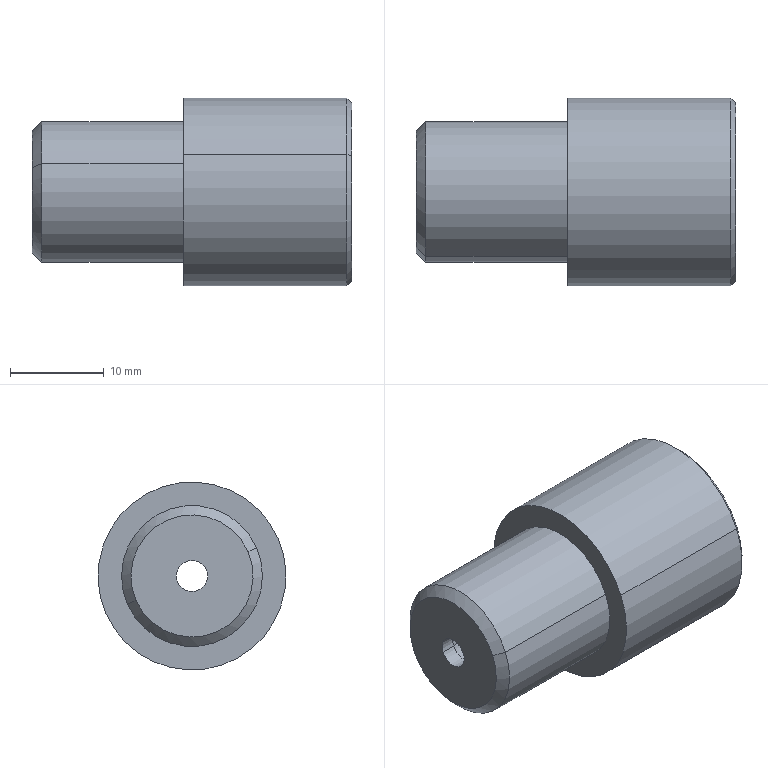Part | STEP file | 35-TOE-IN(B35) | 1 solid | 21 faces | box 34 x 20 x 20 mm | volume 6255 mm3 | cylinder 8 | cone 6 | sphere 4 | plane 3 | commonest cylinder face diameters 3.32 x2 10 x2 15 x2 20 x2